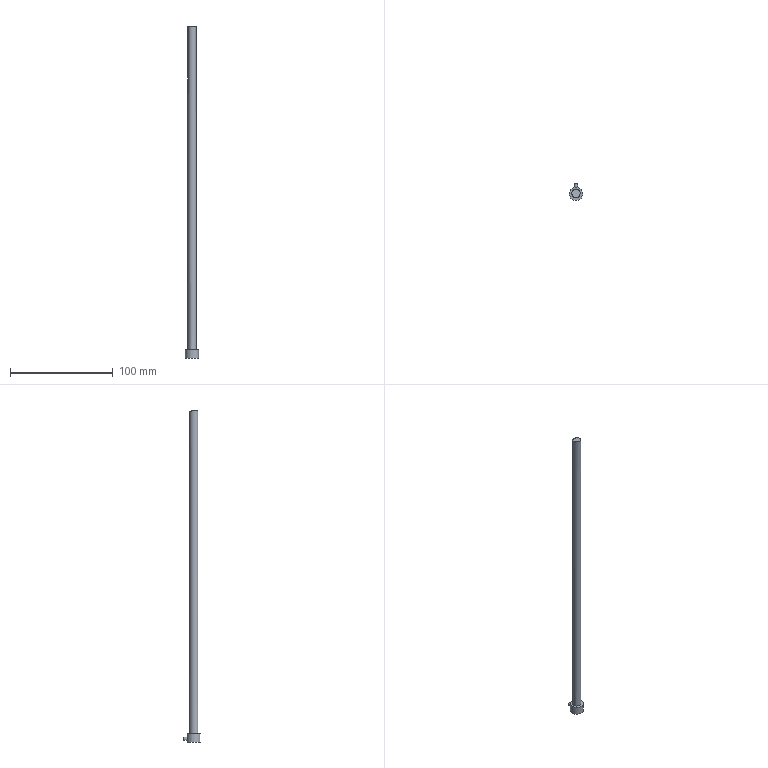Part | STEP file | E108-04-325 | 1 solid | 8 faces | box 13 x 16.5 x 322.523 mm | volume 16862 mm3 | cylinder 3 | plane 3 | spline 1 | cone 1 | commonest cylinder face diameters 3 x1 8 x1 13 x1
STEP:
#1=CARTESIAN_POINT('',(0.,0.,0.));
#2=DIRECTION('',(0.,0.,1.));
#3=DIRECTION('',(1.,0.,0.));
#4=AXIS2_PLACEMENT_3D('',#1,#2,#3);
#5=CARTESIAN_POINT('',(-1.397,3.748,321.27));
#6=VERTEX_POINT('',#5);
#7=CARTESIAN_POINT('',(-1.397,3.748,321.27));
#8=CARTESIAN_POINT('',(-1.815,3.592,321.278));
#9=CARTESIAN_POINT('',(-2.211,3.363,321.295));
#10=CARTESIAN_POINT('',(-2.554,3.079,321.322));
#11=CARTESIAN_POINT('',(-2.896,2.795,321.348));
#12=CARTESIAN_POINT('',(-3.194,2.449,321.384));
#13=CARTESIAN_POINT('',(-3.423,2.069,321.427));
#14=CARTESIAN_POINT('',(-3.653,1.688,321.472));
#15=CARTESIAN_POINT('',(-3.821,1.264,321.525));
#16=CARTESIAN_POINT('',(-3.913,0.83,321.584));
#17=CARTESIAN_POINT('',(-4.006,0.3925,321.644));
#18=CARTESIAN_POINT('',(-4.024,-0.06598,321.712));
#19=CARTESIAN_POINT('',(-3.968,-0.5081,321.783));
#20=CARTESIAN_POINT('',(-3.91,-0.955,321.854));
#21=CARTESIAN_POINT('',(-3.775,-1.397,321.93));
#22=CARTESIAN_POINT('',(-3.572,-1.8,322.004));
#23=CARTESIAN_POINT('',(-3.368,-2.204,322.078));
#24=CARTESIAN_POINT('',(-3.091,-2.58,322.152));
#25=CARTESIAN_POINT('',(-2.762,-2.893,322.219));
#26=CARTESIAN_POINT('',(-2.434,-3.207,322.285));
#27=CARTESIAN_POINT('',(-2.046,-3.467,322.346));
#28=CARTESIAN_POINT('',(-1.629,-3.653,322.394));
#29=CARTESIAN_POINT('',(-1.219,-3.836,322.442));
#30=CARTESIAN_POINT('',(-0.7694,-3.951,322.478));
#31=CARTESIAN_POINT('',(-0.3192,-3.987,322.499));
#32=CARTESIAN_POINT('',(0.123,-4.023,322.52));
#33=CARTESIAN_POINT('',(0.5783,-3.983,322.527));
#34=CARTESIAN_POINT('',(1.008,-3.871,322.519));
#35=CARTESIAN_POINT('',(1.434,-3.76,322.512));
#36=CARTESIAN_POINT('',(1.846,-3.576,322.489));
#37=CARTESIAN_POINT('',(2.211,-3.333,322.455));
#38=CARTESIAN_POINT('',(2.578,-3.09,322.421));
#39=CARTESIAN_POINT('',(2.907,-2.782,322.374));
#40=CARTESIAN_POINT('',(3.174,-2.434,322.319));
#41=CARTESIAN_POINT('',(3.444,-2.082,322.264));
#42=CARTESIAN_POINT('',(3.657,-1.679,322.199));
#43=CARTESIAN_POINT('',(3.797,-1.259,322.132));
#44=CARTESIAN_POINT('',(3.938,-0.8318,322.064));
#45=CARTESIAN_POINT('',(4.008,-0.3752,321.991));
#46=CARTESIAN_POINT('',(3.999,0.07396,321.92));
#47=CARTESIAN_POINT('',(3.991,0.5268,321.849));
#48=CARTESIAN_POINT('',(3.903,0.9847,321.778));
#49=CARTESIAN_POINT('',(3.743,1.409,321.712));
#50=CARTESIAN_POINT('',(3.584,1.833,321.647));
#51=CARTESIAN_POINT('',(3.348,2.236,321.585));
#52=CARTESIAN_POINT('',(3.054,2.583,321.531));
#53=CARTESIAN_POINT('',(2.763,2.928,321.478));
#54=CARTESIAN_POINT('',(2.406,3.227,321.431));
#55=CARTESIAN_POINT('',(2.015,3.455,321.393));
#56=CARTESIAN_POINT('',(1.628,3.681,321.355));
#57=CARTESIAN_POINT('',(1.195,3.844,321.324));
#58=CARTESIAN_POINT('',(0.7533,3.928,321.303));
#59=CARTESIAN_POINT('',(0.3148,4.013,321.282));
#60=CARTESIAN_POINT('',(-0.1448,4.022,321.27));
#61=CARTESIAN_POINT('',(-0.587,3.957,321.266));
#62=CARTESIAN_POINT('',(-0.8629,3.916,321.264));
#63=CARTESIAN_POINT('',(-1.136,3.845,321.265));
#64=CARTESIAN_POINT('',(-1.397,3.748,321.27));
#65=B_SPLINE_CURVE_WITH_KNOTS('',3,(#7,#8,#9,#10,#11,#12,#13,#14,#15,#16,#17,#18,#19,#20,#21,#22,#23,#24,#25,#26,#27,#28,#29,#30,#31,#32,#33,#34,#35,#36,#37,#38,#39,#40,#41,#42,#43,#44,#45,#46,#47,#48,#49,#50,#51,#52,#53,#54,#55,#56,#57,#58,#59,#60,#61,#62,#63,#64),.UNSPECIFIED.,.T.,.F.,(1,3,3,3,3,3,3,3,3,3,3,3,3,3,3,3,3,3,3,3,3,1),(-0.03296,0.,0.05312,0.1062,0.1595,0.2133,0.2677,0.3225,0.3772,0.4311,0.484,0.5364,0.589,0.6424,0.6966,0.7513,0.8059,0.8601,0.9138,0.967,1.,1.053),.UNSPECIFIED.);
#66=CARTESIAN_POINT('',(0.,0.,108.));
#67=DIRECTION('',(0.,0.,-1.));
#68=DIRECTION('',(-1.,0.,0.));
#69=AXIS2_PLACEMENT_3D('',#66,#67,#68);
#70=CYLINDRICAL_SURFACE('',#69,4.);
#71=CARTESIAN_POINT('',(7.497,-213.27));
#72=CARTESIAN_POINT('',(7.473,-213.272));
#73=CARTESIAN_POINT('',(7.426,-213.276));
#74=CARTESIAN_POINT('',(7.354,-213.285));
#75=CARTESIAN_POINT('',(7.282,-213.297));
#76=CARTESIAN_POINT('',(7.21,-213.31));
#77=CARTESIAN_POINT('',(7.138,-213.327));
#78=CARTESIAN_POINT('',(7.067,-213.346));
#79=CARTESIAN_POINT('',(6.995,-213.367));
#80=CARTESIAN_POINT('',(6.923,-213.391));
#81=CARTESIAN_POINT('',(6.852,-213.417));
#82=CARTESIAN_POINT('',(6.781,-213.446));
#83=CARTESIAN_POINT('',(6.709,-213.477));
#84=CARTESIAN_POINT('',(6.637,-213.51));
#85=CARTESIAN_POINT('',(6.566,-213.545));
#86=CARTESIAN_POINT('',(6.495,-213.583));
#87=CARTESIAN_POINT('',(6.424,-213.622));
#88=CARTESIAN_POINT('',(6.353,-213.662));
#89=CARTESIAN_POINT('',(6.282,-213.705));
#90=CARTESIAN_POINT('',(6.21,-213.748));
#91=CARTESIAN_POINT('',(6.14,-213.793));
#92=CARTESIAN_POINT('',(6.069,-213.838));
#93=CARTESIAN_POINT('',(5.998,-213.884));
#94=CARTESIAN_POINT('',(5.927,-213.931));
#95=CARTESIAN_POINT('',(5.856,-213.978));
#96=CARTESIAN_POINT('',(5.785,-214.024));
#97=CARTESIAN_POINT('',(5.715,-214.07));
#98=CARTESIAN_POINT('',(5.643,-214.116));
#99=CARTESIAN_POINT('',(5.572,-214.16));
#100=CARTESIAN_POINT('',(5.501,-214.203));
#101=CARTESIAN_POINT('',(5.431,-214.244));
#102=CARTESIAN_POINT('',(5.359,-214.284));
#103=CARTESIAN_POINT('',(5.288,-214.322));
#104=CARTESIAN_POINT('',(5.217,-214.357));
#105=CARTESIAN_POINT('',(5.145,-214.389));
#106=CARTESIAN_POINT('',(5.074,-214.418));
#107=CARTESIAN_POINT('',(5.003,-214.444));
#108=CARTESIAN_POINT('',(4.931,-214.467));
#109=CARTESIAN_POINT('',(4.859,-214.486));
#110=CARTESIAN_POINT('',(4.788,-214.501));
#111=CARTESIAN_POINT('',(4.716,-214.512));
#112=CARTESIAN_POINT('',(4.644,-214.52));
#113=CARTESIAN_POINT('',(4.572,-214.523));
#114=CARTESIAN_POINT('',(4.5,-214.522));
#115=CARTESIAN_POINT('',(4.429,-214.518));
#116=CARTESIAN_POINT('',(4.357,-214.509));
#117=CARTESIAN_POINT('',(4.285,-214.496));
#118=CARTESIAN_POINT('',(4.213,-214.48));
#119=CARTESIAN_POINT('',(4.141,-214.46));
#120=CARTESIAN_POINT('',(4.07,-214.437));
#121=CARTESIAN_POINT('',(3.998,-214.41));
#122=CARTESIAN_POINT('',(3.927,-214.381));
#123=CARTESIAN_POINT('',(3.855,-214.348));
#124=CARTESIAN_POINT('',(3.784,-214.314));
#125=CARTESIAN_POINT('',(3.713,-214.277));
#126=CARTESIAN_POINT('',(3.642,-214.238));
#127=CARTESIAN_POINT('',(3.57,-214.197));
#128=CARTESIAN_POINT('',(3.499,-214.155));
#129=CARTESIAN_POINT('',(3.429,-214.112));
#130=CARTESIAN_POINT('',(3.358,-214.068));
#131=CARTESIAN_POINT('',(3.286,-214.024));
#132=CARTESIAN_POINT('',(3.215,-213.979));
#133=CARTESIAN_POINT('',(3.144,-213.934));
#134=CARTESIAN_POINT('',(3.074,-213.889));
#135=CARTESIAN_POINT('',(3.003,-213.845));
#136=CARTESIAN_POINT('',(2.932,-213.801));
#137=CARTESIAN_POINT('',(2.86,-213.758));
#138=CARTESIAN_POINT('',(2.79,-213.717));
#139=CARTESIAN_POINT('',(2.719,-213.676));
#140=CARTESIAN_POINT('',(2.647,-213.637));
#141=CARTESIAN_POINT('',(2.576,-213.599));
#142=CARTESIAN_POINT('',(2.505,-213.563));
#143=CARTESIAN_POINT('',(2.434,-213.528));
#144=CARTESIAN_POINT('',(2.362,-213.496));
#145=CARTESIAN_POINT('',(2.291,-213.465));
#146=CARTESIAN_POINT('',(2.219,-213.436));
#147=CARTESIAN_POINT('',(2.148,-213.409));
#148=CARTESIAN_POINT('',(2.076,-213.385));
#149=CARTESIAN_POINT('',(2.005,-213.362));
#150=CARTESIAN_POINT('',(1.933,-213.342));
#151=CARTESIAN_POINT('',(1.861,-213.324));
#152=CARTESIAN_POINT('',(1.79,-213.309));
#153=CARTESIAN_POINT('',(1.718,-213.295));
#154=CARTESIAN_POINT('',(1.646,-213.284));
#155=CARTESIAN_POINT('',(1.574,-213.276));
#156=CARTESIAN_POINT('',(1.502,-213.27));
#157=CARTESIAN_POINT('',(1.431,-213.266));
#158=CARTESIAN_POINT('',(1.359,-213.265));
#159=CARTESIAN_POINT('',(1.286,-213.266));
#160=CARTESIAN_POINT('',(1.238,-213.269));
#161=CARTESIAN_POINT('',(1.214,-213.27));
#162=B_SPLINE_CURVE_WITH_KNOTS('',3,(#71,#72,#73,#74,#75,#76,#77,#78,#79,#80,#81,#82,#83,#84,#85,#86,#87,#88,#89,#90,#91,#92,#93,#94,#95,#96,#97,#98,#99,#100,#101,#102,#103,#104,#105,#106,#107,#108,#109,#110,#111,#112,#113,#114,#115,#116,#117,#118,#119,#120,#121,#122,#123,#124,#125,#126,#127,#128,#129,#130,#131,#132,#133,#134,#135,#136,#137,#138,#139,#140,#141,#142,#143,#144,#145,#146,#147,#148,#149,#150,#151,#152,#153,#154,#155,#156,#157,#158,#159,#160,#161),.UNSPECIFIED.,.F.,.F.,(4,1,1,1,1,1,1,1,1,1,1,1,1,1,1,1,1,1,1,1,1,1,1,1,1,1,1,1,1,1,1,1,1,1,1,1,1,1,1,1,1,1,1,1,1,1,1,1,1,1,1,1,1,1,1,1,1,1,1,1,1,1,1,1,1,1,1,1,1,1,1,1,1,1,1,1,1,1,1,1,1,1,1,1,1,1,1,1,4),(0.,0.01136,0.02273,0.03409,0.04545,0.05682,0.06818,0.07955,0.09091,0.1023,0.1136,0.125,0.1364,0.1477,0.1591,0.1705,0.1818,0.1932,0.2045,0.2159,0.2273,0.2386,0.25,0.2614,0.2727,0.2841,0.2955,0.3068,0.3182,0.3295,0.3409,0.3523,0.3636,0.375,0.3864,0.3977,0.4091,0.4205,0.4318,0.4432,0.4545,0.4659,0.4773,0.4886,0.5,0.5114,0.5227,0.5341,0.5455,0.5568,0.5682,0.5795,0.5909,0.6023,0.6136,0.625,0.6364,0.6477,0.6591,0.6705,0.6818,0.6932,0.7045,0.7159,0.7273,0.7386,0.75,0.7614,0.7727,0.7841,0.7955,0.8068,0.8182,0.8295,0.8409,0.8523,0.8636,0.875,0.8864,0.8977,0.9091,0.9205,0.9318,0.9432,0.9545,0.9659,0.9773,0.9886,1.),.QUASI_UNIFORM_KNOTS.);
#163=(GEOMETRIC_REPRESENTATION_CONTEXT(2)PARAMETRIC_REPRESENTATION_CONTEXT()REPRESENTATION_CONTEXT('',''));
#164=DEFINITIONAL_REPRESENTATION('',(#162),#163);
#165=PCURVE('',#70,#164);
#166=CARTESIAN_POINT('',(19.927,-1.061,321.866));
#167=CARTESIAN_POINT('',(18.638,5.204,320.799));
#168=CARTESIAN_POINT('',(17.382,11.513,320.097));
#169=CARTESIAN_POINT('',(16.146,17.876,319.645));
#170=CARTESIAN_POINT('',(13.703,-2.125,322.326));
#171=CARTESIAN_POINT('',(12.375,4.073,321.242));
#172=CARTESIAN_POINT('',(11.072,10.308,320.518));
#173=CARTESIAN_POINT('',(9.785,16.592,320.042));
#174=CARTESIAN_POINT('',(7.218,-3.361,322.621));
#175=CARTESIAN_POINT('',(5.852,2.773,321.508));
#176=CARTESIAN_POINT('',(4.506,8.942,320.75));
#177=CARTESIAN_POINT('',(3.17,15.156,320.239));
#178=CARTESIAN_POINT('',(-6.604,-6.202,322.705));
#179=CARTESIAN_POINT('',(-8.034,-0.1978,321.507));
#180=CARTESIAN_POINT('',(-9.458,5.839,320.656));
#181=CARTESIAN_POINT('',(-10.883,11.916,320.054));
#182=CARTESIAN_POINT('',(-13.939,-7.81,322.49));
#183=CARTESIAN_POINT('',(-15.395,-1.87,321.235));
#184=CARTESIAN_POINT('',(-16.854,4.101,320.327));
#185=CARTESIAN_POINT('',(-18.32,10.11,319.669));
#186=CARTESIAN_POINT('',(-29.513,-11.391,321.285));
#187=CARTESIAN_POINT('',(-31.002,-5.589,319.888));
#188=CARTESIAN_POINT('',(-32.516,0.2464,318.841));
#189=CARTESIAN_POINT('',(-34.052,6.11,318.053));
#190=CARTESIAN_POINT('',(-37.747,-13.364,320.293));
#191=CARTESIAN_POINT('',(-39.245,-7.634,318.809));
#192=CARTESIAN_POINT('',(-40.779,-1.871,317.681));
#193=CARTESIAN_POINT('',(-42.344,3.916,316.819));
#194=CARTESIAN_POINT('',(-54.974,-17.604,317.285));
#195=CARTESIAN_POINT('',(-56.464,-12.039,315.613));
#196=CARTESIAN_POINT('',(-58.018,-6.437,314.309));
#197=CARTESIAN_POINT('',(-59.625,-0.8214,313.287));
#198=CARTESIAN_POINT('',(-63.963,-19.87,315.268));
#199=CARTESIAN_POINT('',(-65.438,-14.397,313.494));
#200=CARTESIAN_POINT('',(-66.991,-8.885,312.095));
#201=CARTESIAN_POINT('',(-68.61,-3.364,310.987));
#202=CARTESIAN_POINT('',(-73.219,-22.228,312.641));
#203=CARTESIAN_POINT('',(-74.668,-16.858,310.779));
#204=CARTESIAN_POINT('',(-76.208,-11.45,309.295));
#205=CARTESIAN_POINT('',(-77.828,-6.035,308.108));
#206=B_SPLINE_SURFACE_WITH_KNOTS('',3,3,((#166,#167,#168,#169),(#170,#171,#172,#173),(#174,#175,#176,#177),(#178,#179,#180,#181),(#182,#183,#184,#185),(#186,#187,#188,#189),(#190,#191,#192,#193),(#194,#195,#196,#197),(#198,#199,#200,#201),(#202,#203,#204,#205)),.UNSPECIFIED.,.F.,.F.,.F.,(4,2,2,2,4),(4,4),(0.,0.25,0.5,0.75,1.),(0.,1.),.UNSPECIFIED.);
#207=CARTESIAN_POINT('',(0.2472,0.4644));
#208=CARTESIAN_POINT('',(0.2483,0.4637));
#209=CARTESIAN_POINT('',(0.2505,0.4619));
#210=CARTESIAN_POINT('',(0.2538,0.458));
#211=CARTESIAN_POINT('',(0.257,0.4532));
#212=CARTESIAN_POINT('',(0.2601,0.4473));
#213=CARTESIAN_POINT('',(0.2631,0.4405));
#214=CARTESIAN_POINT('',(0.2659,0.4326));
#215=CARTESIAN_POINT('',(0.2687,0.4239));
#216=CARTESIAN_POINT('',(0.2713,0.4142));
#217=CARTESIAN_POINT('',(0.2738,0.4038));
#218=CARTESIAN_POINT('',(0.276,0.3926));
#219=CARTESIAN_POINT('',(0.2781,0.3807));
#220=CARTESIAN_POINT('',(0.28,0.3681));
#221=CARTESIAN_POINT('',(0.2817,0.3549));
#222=CARTESIAN_POINT('',(0.2833,0.3413));
#223=CARTESIAN_POINT('',(0.2845,0.3272));
#224=CARTESIAN_POINT('',(0.2856,0.3127));
#225=CARTESIAN_POINT('',(0.2865,0.2979));
#226=CARTESIAN_POINT('',(0.2871,0.2829));
#227=CARTESIAN_POINT('',(0.2875,0.2679));
#228=CARTESIAN_POINT('',(0.2876,0.2527));
#229=CARTESIAN_POINT('',(0.2876,0.2374));
#230=CARTESIAN_POINT('',(0.2873,0.2223));
#231=CARTESIAN_POINT('',(0.2867,0.2073));
#232=CARTESIAN_POINT('',(0.286,0.1926));
#233=CARTESIAN_POINT('',(0.285,0.1782));
#234=CARTESIAN_POINT('',(0.2838,0.1641));
#235=CARTESIAN_POINT('',(0.2824,0.1505));
#236=CARTESIAN_POINT('',(0.2807,0.1374));
#237=CARTESIAN_POINT('',(0.2789,0.1249));
#238=CARTESIAN_POINT('',(0.2769,0.113));
#239=CARTESIAN_POINT('',(0.2747,0.1018));
#240=CARTESIAN_POINT('',(0.2723,0.0914));
#241=CARTESIAN_POINT('',(0.2697,0.08183));
#242=CARTESIAN_POINT('',(0.267,0.07317));
#243=CARTESIAN_POINT('',(0.2641,0.06539));
#244=CARTESIAN_POINT('',(0.2612,0.05855));
#245=CARTESIAN_POINT('',(0.2581,0.05272));
#246=CARTESIAN_POINT('',(0.2549,0.04796));
#247=CARTESIAN_POINT('',(0.2516,0.04427));
#248=CARTESIAN_POINT('',(0.2483,0.04165));
#249=CARTESIAN_POINT('',(0.2449,0.04012));
#250=CARTESIAN_POINT('',(0.2415,0.0397));
#251=CARTESIAN_POINT('',(0.2381,0.04039));
#252=CARTESIAN_POINT('',(0.2347,0.0422));
#253=CARTESIAN_POINT('',(0.2313,0.04511));
#254=CARTESIAN_POINT('',(0.228,0.04908));
#255=CARTESIAN_POINT('',(0.2247,0.05408));
#256=CARTESIAN_POINT('',(0.2216,0.06009));
#257=CARTESIAN_POINT('',(0.2185,0.06713));
#258=CARTESIAN_POINT('',(0.2155,0.07511));
#259=CARTESIAN_POINT('',(0.2127,0.08397));
#260=CARTESIAN_POINT('',(0.21,0.09363));
#261=CARTESIAN_POINT('',(0.2075,0.1041));
#262=CARTESIAN_POINT('',(0.2051,0.1154));
#263=CARTESIAN_POINT('',(0.2029,0.1273));
#264=CARTESIAN_POINT('',(0.2009,0.1399));
#265=CARTESIAN_POINT('',(0.1992,0.1529));
#266=CARTESIAN_POINT('',(0.1976,0.1665));
#267=CARTESIAN_POINT('',(0.1963,0.1805));
#268=CARTESIAN_POINT('',(0.1952,0.1949));
#269=CARTESIAN_POINT('',(0.1943,0.2096));
#270=CARTESIAN_POINT('',(0.1936,0.2244));
#271=CARTESIAN_POINT('',(0.1933,0.2394));
#272=CARTESIAN_POINT('',(0.1931,0.2545));
#273=CARTESIAN_POINT('',(0.1932,0.2696));
#274=CARTESIAN_POINT('',(0.1935,0.2846));
#275=CARTESIAN_POINT('',(0.1941,0.2993));
#276=CARTESIAN_POINT('',(0.1949,0.314));
#277=CARTESIAN_POINT('',(0.196,0.3283));
#278=CARTESIAN_POINT('',(0.1972,0.3423));
#279=CARTESIAN_POINT('',(0.1987,0.3558));
#280=CARTESIAN_POINT('',(0.2005,0.3688));
#281=CARTESIAN_POINT('',(0.2024,0.3812));
#282=CARTESIAN_POINT('',(0.2045,0.3931));
#283=CARTESIAN_POINT('',(0.2068,0.4042));
#284=CARTESIAN_POINT('',(0.2093,0.4145));
#285=CARTESIAN_POINT('',(0.2119,0.424));
#286=CARTESIAN_POINT('',(0.2147,0.4327));
#287=CARTESIAN_POINT('',(0.2177,0.4405));
#288=CARTESIAN_POINT('',(0.2207,0.4474));
#289=CARTESIAN_POINT('',(0.2238,0.4532));
#290=CARTESIAN_POINT('',(0.227,0.458));
#291=CARTESIAN_POINT('',(0.2303,0.4618));
#292=CARTESIAN_POINT('',(0.2337,0.4646));
#293=CARTESIAN_POINT('',(0.237,0.4662));
#294=CARTESIAN_POINT('',(0.2404,0.4668));
#295=CARTESIAN_POINT('',(0.2438,0.4662));
#296=CARTESIAN_POINT('',(0.2461,0.4651));
#297=CARTESIAN_POINT('',(0.2472,0.4644));
#298=B_SPLINE_CURVE_WITH_KNOTS('',3,(#207,#208,#209,#210,#211,#212,#213,#214,#215,#216,#217,#218,#219,#220,#221,#222,#223,#224,#225,#226,#227,#228,#229,#230,#231,#232,#233,#234,#235,#236,#237,#238,#239,#240,#241,#242,#243,#244,#245,#246,#247,#248,#249,#250,#251,#252,#253,#254,#255,#256,#257,#258,#259,#260,#261,#262,#263,#264,#265,#266,#267,#268,#269,#270,#271,#272,#273,#274,#275,#276,#277,#278,#279,#280,#281,#282,#283,#284,#285,#286,#287,#288,#289,#290,#291,#292,#293,#294,#295,#296,#297),.UNSPECIFIED.,.T.,.F.,(4,1,1,1,1,1,1,1,1,1,1,1,1,1,1,1,1,1,1,1,1,1,1,1,1,1,1,1,1,1,1,1,1,1,1,1,1,1,1,1,1,1,1,1,1,1,1,1,1,1,1,1,1,1,1,1,1,1,1,1,1,1,1,1,1,1,1,1,1,1,1,1,1,1,1,1,1,1,1,1,1,1,1,1,1,1,1,1,4),(0.,0.01136,0.02273,0.03409,0.04545,0.05682,0.06818,0.07955,0.09091,0.1023,0.1136,0.125,0.1364,0.1477,0.1591,0.1705,0.1818,0.1932,0.2045,0.2159,0.2273,0.2386,0.25,0.2614,0.2727,0.2841,0.2955,0.3068,0.3182,0.3295,0.3409,0.3523,0.3636,0.375,0.3864,0.3977,0.4091,0.4205,0.4318,0.4432,0.4545,0.4659,0.4773,0.4886,0.5,0.5114,0.5227,0.5341,0.5455,0.5568,0.5682,0.5795,0.5909,0.6023,0.6136,0.625,0.6364,0.6477,0.6591,0.6705,0.6818,0.6932,0.7045,0.7159,0.7273,0.7386,0.75,0.7614,0.7727,0.7841,0.7955,0.8068,0.8182,0.8295,0.8409,0.8523,0.8636,0.875,0.8864,0.8977,0.9091,0.9205,0.9318,0.9432,0.9545,0.9659,0.9773,0.9886,1.),.QUASI_UNIFORM_KNOTS.);
#299=(GEOMETRIC_REPRESENTATION_CONTEXT(2)PARAMETRIC_REPRESENTATION_CONTEXT()REPRESENTATION_CONTEXT('',''));
#300=DEFINITIONAL_REPRESENTATION('',(#298),#299);
#301=PCURVE('',#206,#300);
#302=SURFACE_CURVE('',#65,(#165,#301),.PCURVE_S1.);
#303=EDGE_CURVE('',#6,#6,#302,.T.);
#304=ORIENTED_EDGE('',*,*,#303,.F.);
#305=CARTESIAN_POINT('',(-1.397,3.748,8.));
#306=VERTEX_POINT('',#305);
#307=CARTESIAN_POINT('',(-1.397,3.748,321.27));
#308=CARTESIAN_POINT('',(-1.397,3.748,8.));
#309=B_SPLINE_CURVE_WITH_KNOTS('',1,(#307,#308),.UNSPECIFIED.,.F.,.F.,(2,2),(-213.27,100.),.PIECEWISE_BEZIER_KNOTS.);
#310=CARTESIAN_POINT('',(7.497,0.));
#311=DIRECTION('',(0.,1.));
#312=VECTOR('',#311,1.);
#313=LINE('',#310,#312);
#314=(GEOMETRIC_REPRESENTATION_CONTEXT(2)PARAMETRIC_REPRESENTATION_CONTEXT()REPRESENTATION_CONTEXT('',''));
#315=DEFINITIONAL_REPRESENTATION('',(#313),#314);
#316=PCURVE('',#70,#315);
#317=CARTESIAN_POINT('',(1.214,0.));
#318=DIRECTION('',(0.,1.));
#319=VECTOR('',#318,1.);
#320=LINE('',#317,#319);
#321=(GEOMETRIC_REPRESENTATION_CONTEXT(2)PARAMETRIC_REPRESENTATION_CONTEXT()REPRESENTATION_CONTEXT('',''));
#322=DEFINITIONAL_REPRESENTATION('',(#320),#321);
#323=PCURVE('',#70,#322);
#324=SEAM_CURVE('',#309,(#316,#323),.PCURVE_S1.);
#325=EDGE_CURVE('',#6,#306,#324,.T.);
#326=ORIENTED_EDGE('',*,*,#325,.T.);
#327=CARTESIAN_POINT('',(4.,0.,8.));
#328=VERTEX_POINT('',#327);
#329=CARTESIAN_POINT('',(0.,0.,8.));
#330=DIRECTION('',(0.,0.,1.));
#331=DIRECTION('',(1.,0.,0.));
#332=AXIS2_PLACEMENT_3D('',#329,#330,#331);
#333=CIRCLE('',#332,4.);
#334=CARTESIAN_POINT('',(9.425,100.));
#335=DIRECTION('',(-1.,0.));
#336=VECTOR('',#335,1.);
#337=LINE('',#334,#336);
#338=(GEOMETRIC_REPRESENTATION_CONTEXT(2)PARAMETRIC_REPRESENTATION_CONTEXT()REPRESENTATION_CONTEXT('',''));
#339=DEFINITIONAL_REPRESENTATION('',(#337),#338);
#340=PCURVE('',#70,#339);
#341=CARTESIAN_POINT('',(0.,0.,8.));
#342=DIRECTION('',(0.,0.,-1.));
#343=DIRECTION('',(1.,0.,0.));
#344=AXIS2_PLACEMENT_3D('',#341,#342,#343);
#345=PLANE('',#344);
#346=CARTESIAN_POINT('',(4.,0.));
#347=CARTESIAN_POINT('',(4.,-6.928));
#348=CARTESIAN_POINT('',(-2.,-3.464));
#349=CARTESIAN_POINT('',(-8.,0.));
#350=CARTESIAN_POINT('',(-2.,3.464));
#351=CARTESIAN_POINT('',(4.,6.928));
#352=CARTESIAN_POINT('',(4.,0.));
#353=(BOUNDED_CURVE()B_SPLINE_CURVE(2,(#346,#347,#348,#349,#350,#351,#352),.UNSPECIFIED.,.T.,.F.)B_SPLINE_CURVE_WITH_KNOTS((1,2,2,2,2,1),(-2.094,0.,2.094,4.189,6.283,8.378),.UNSPECIFIED.)CURVE()GEOMETRIC_REPRESENTATION_ITEM()RATIONAL_B_SPLINE_CURVE((1.,0.5,1.,0.5,1.,0.5,1.))REPRESENTATION_ITEM(''));
#354=(GEOMETRIC_REPRESENTATION_CONTEXT(2)PARAMETRIC_REPRESENTATION_CONTEXT()REPRESENTATION_CONTEXT('',''));
#355=DEFINITIONAL_REPRESENTATION('',(#353),#354);
#356=PCURVE('',#345,#355);
#357=SURFACE_CURVE('',#333,(#340,#356),.PCURVE_S1.);
#358=EDGE_CURVE('',#306,#328,#357,.T.);
#359=ORIENTED_EDGE('',*,*,#358,.T.);
#360=CARTESIAN_POINT('',(0.,0.,8.));
#361=DIRECTION('',(0.,0.,1.));
#362=DIRECTION('',(1.,0.,0.));
#363=AXIS2_PLACEMENT_3D('',#360,#361,#362);
#364=CIRCLE('',#363,4.);
#365=CARTESIAN_POINT('',(3.142,100.));
#366=DIRECTION('',(-1.,0.));
#367=VECTOR('',#366,1.);
#368=LINE('',#365,#367);
#369=(GEOMETRIC_REPRESENTATION_CONTEXT(2)PARAMETRIC_REPRESENTATION_CONTEXT()REPRESENTATION_CONTEXT('',''));
#370=DEFINITIONAL_REPRESENTATION('',(#368),#369);
#371=PCURVE('',#70,#370);
#372=CARTESIAN_POINT('',(4.,0.));
#373=CARTESIAN_POINT('',(4.,-6.928));
#374=CARTESIAN_POINT('',(-2.,-3.464));
#375=CARTESIAN_POINT('',(-8.,0.));
#376=CARTESIAN_POINT('',(-2.,3.464));
#377=CARTESIAN_POINT('',(4.,6.928));
#378=CARTESIAN_POINT('',(4.,0.));
#379=(BOUNDED_CURVE()B_SPLINE_CURVE(2,(#372,#373,#374,#375,#376,#377,#378),.UNSPECIFIED.,.T.,.F.)B_SPLINE_CURVE_WITH_KNOTS((1,2,2,2,2,1),(-2.094,0.,2.094,4.189,6.283,8.378),.UNSPECIFIED.)CURVE()GEOMETRIC_REPRESENTATION_ITEM()RATIONAL_B_SPLINE_CURVE((1.,0.5,1.,0.5,1.,0.5,1.))REPRESENTATION_ITEM(''));
#380=(GEOMETRIC_REPRESENTATION_CONTEXT(2)PARAMETRIC_REPRESENTATION_CONTEXT()REPRESENTATION_CONTEXT('',''));
#381=DEFINITIONAL_REPRESENTATION('',(#379),#380);
#382=PCURVE('',#345,#381);
#383=SURFACE_CURVE('',#364,(#371,#382),.PCURVE_S1.);
#384=EDGE_CURVE('',#328,#306,#383,.T.);
#385=ORIENTED_EDGE('',*,*,#384,.T.);
#386=ORIENTED_EDGE('',*,*,#325,.F.);
#387=EDGE_LOOP('',(#304,#326,#359,#385,#386));
#388=FACE_BOUND('',#387,.T.);
#389=ADVANCED_FACE('',(#388),#70,.T.);
#390=ORIENTED_EDGE('',*,*,#303,.F.);
#391=EDGE_LOOP('',(#390));
#392=FACE_BOUND('',#391,.F.);
#393=ADVANCED_FACE('',(#392),#206,.F.);
#394=CARTESIAN_POINT('',(6.5,0.,0.));
#395=VERTEX_POINT('',#394);
#396=CARTESIAN_POINT('',(-6.5,0.,0.));
#397=VERTEX_POINT('',#396);
#398=CARTESIAN_POINT('',(0.,0.,0.));
#399=DIRECTION('',(0.,0.,-1.));
#400=DIRECTION('',(-1.,0.,0.));
#401=AXIS2_PLACEMENT_3D('',#398,#399,#400);
#402=CIRCLE('',#401,6.5);
#403=CARTESIAN_POINT('',(0.,0.,8.));
#404=DIRECTION('',(0.,0.,-1.));
#405=DIRECTION('',(1.,0.,0.));
#406=AXIS2_PLACEMENT_3D('',#403,#404,#405);
#407=CYLINDRICAL_SURFACE('',#406,6.5);
#408=CARTESIAN_POINT('',(-3.142,8.));
#409=DIRECTION('',(1.,0.));
#410=VECTOR('',#409,1.);
#411=LINE('',#408,#410);
#412=(GEOMETRIC_REPRESENTATION_CONTEXT(2)PARAMETRIC_REPRESENTATION_CONTEXT()REPRESENTATION_CONTEXT('',''));
#413=DEFINITIONAL_REPRESENTATION('',(#411),#412);
#414=PCURVE('',#407,#413);
#415=CARTESIAN_POINT('',(240.,-1000.,0.));
#416=DIRECTION('',(0.,0.,1.));
#417=DIRECTION('',(-1.,0.,0.));
#418=AXIS2_PLACEMENT_3D('',#415,#416,#417);
#419=PLANE('',#418);
#420=CARTESIAN_POINT('',(246.5,-1000.));
#421=CARTESIAN_POINT('',(246.5,-1011.258));
#422=CARTESIAN_POINT('',(236.75,-1005.629));
#423=CARTESIAN_POINT('',(227.,-1000.));
#424=CARTESIAN_POINT('',(236.75,-994.371));
#425=CARTESIAN_POINT('',(246.5,-988.742));
#426=CARTESIAN_POINT('',(246.5,-1000.));
#427=(BOUNDED_CURVE()B_SPLINE_CURVE(2,(#420,#421,#422,#423,#424,#425,#426),.UNSPECIFIED.,.T.,.F.)B_SPLINE_CURVE_WITH_KNOTS((1,2,2,2,2,1),(-2.094,0.,2.094,4.189,6.283,8.378),.UNSPECIFIED.)CURVE()GEOMETRIC_REPRESENTATION_ITEM()RATIONAL_B_SPLINE_CURVE((1.,0.5,1.,0.5,1.,0.5,1.))REPRESENTATION_ITEM(''));
#428=(GEOMETRIC_REPRESENTATION_CONTEXT(2)PARAMETRIC_REPRESENTATION_CONTEXT()REPRESENTATION_CONTEXT('',''));
#429=DEFINITIONAL_REPRESENTATION('',(#427),#428);
#430=PCURVE('',#419,#429);
#431=SURFACE_CURVE('',#402,(#414,#430),.PCURVE_S1.);
#432=EDGE_CURVE('',#395,#397,#431,.T.);
#433=ORIENTED_EDGE('',*,*,#432,.F.);
#434=CARTESIAN_POINT('',(6.5,0.,8.));
#435=VERTEX_POINT('',#434);
#436=CARTESIAN_POINT('',(6.5,0.,8.));
#437=CARTESIAN_POINT('',(6.5,0.,0.));
#438=B_SPLINE_CURVE_WITH_KNOTS('',1,(#436,#437),.UNSPECIFIED.,.F.,.F.,(2,2),(0.,8.),.PIECEWISE_BEZIER_KNOTS.);
#439=CARTESIAN_POINT('',(0.,0.));
#440=DIRECTION('',(0.,1.));
#441=VECTOR('',#440,1.);
#442=LINE('',#439,#441);
#443=(GEOMETRIC_REPRESENTATION_CONTEXT(2)PARAMETRIC_REPRESENTATION_CONTEXT()REPRESENTATION_CONTEXT('',''));
#444=DEFINITIONAL_REPRESENTATION('',(#442),#443);
#445=PCURVE('',#407,#444);
#446=CARTESIAN_POINT('',(6.283,0.));
#447=DIRECTION('',(0.,1.));
#448=VECTOR('',#447,1.);
#449=LINE('',#446,#448);
#450=(GEOMETRIC_REPRESENTATION_CONTEXT(2)PARAMETRIC_REPRESENTATION_CONTEXT()REPRESENTATION_CONTEXT('',''));
#451=DEFINITIONAL_REPRESENTATION('',(#449),#450);
#452=PCURVE('',#407,#451);
#453=SEAM_CURVE('',#438,(#445,#452),.PCURVE_S1.);
#454=EDGE_CURVE('',#435,#395,#453,.T.);
#455=ORIENTED_EDGE('',*,*,#454,.F.);
#456=CARTESIAN_POINT('',(0.,0.,8.));
#457=DIRECTION('',(0.,0.,-1.));
#458=DIRECTION('',(1.,0.,0.));
#459=AXIS2_PLACEMENT_3D('',#456,#457,#458);
#460=CIRCLE('',#459,6.5);
#461=CARTESIAN_POINT('',(0.,0.));
#462=DIRECTION('',(1.,0.));
#463=VECTOR('',#462,1.);
#464=LINE('',#461,#463);
#465=(GEOMETRIC_REPRESENTATION_CONTEXT(2)PARAMETRIC_REPRESENTATION_CONTEXT()REPRESENTATION_CONTEXT('',''));
#466=DEFINITIONAL_REPRESENTATION('',(#464),#465);
#467=PCURVE('',#407,#466);
#468=CARTESIAN_POINT('',(0.,0.));
#469=DIRECTION('',(1.,0.));
#470=AXIS2_PLACEMENT_2D('',#468,#469);
#471=CIRCLE('',#470,6.5);
#472=(GEOMETRIC_REPRESENTATION_CONTEXT(2)PARAMETRIC_REPRESENTATION_CONTEXT()REPRESENTATION_CONTEXT('',''));
#473=DEFINITIONAL_REPRESENTATION('',(#471),#472);
#474=PCURVE('',#345,#473);
#475=SURFACE_CURVE('',#460,(#467,#474),.PCURVE_S1.);
#476=EDGE_CURVE('',#435,#435,#475,.T.);
#477=ORIENTED_EDGE('',*,*,#476,.T.);
#478=ORIENTED_EDGE('',*,*,#454,.T.);
#479=CARTESIAN_POINT('',(0.,0.,0.));
#480=DIRECTION('',(0.,0.,-1.));
#481=DIRECTION('',(-1.,0.,0.));
#482=AXIS2_PLACEMENT_3D('',#479,#480,#481);
#483=CIRCLE('',#482,6.5);
#484=CARTESIAN_POINT('',(3.142,8.));
#485=DIRECTION('',(1.,0.));
#486=VECTOR('',#485,1.);
#487=LINE('',#484,#486);
#488=(GEOMETRIC_REPRESENTATION_CONTEXT(2)PARAMETRIC_REPRESENTATION_CONTEXT()REPRESENTATION_CONTEXT('',''));
#489=DEFINITIONAL_REPRESENTATION('',(#487),#488);
#490=PCURVE('',#407,#489);
#491=CARTESIAN_POINT('',(246.5,-1000.));
#492=CARTESIAN_POINT('',(246.5,-1011.258));
#493=CARTESIAN_POINT('',(236.75,-1005.629));
#494=CARTESIAN_POINT('',(227.,-1000.));
#495=CARTESIAN_POINT('',(236.75,-994.371));
#496=CARTESIAN_POINT('',(246.5,-988.742));
#497=CARTESIAN_POINT('',(246.5,-1000.));
#498=(BOUNDED_CURVE()B_SPLINE_CURVE(2,(#491,#492,#493,#494,#495,#496,#497),.UNSPECIFIED.,.T.,.F.)B_SPLINE_CURVE_WITH_KNOTS((1,2,2,2,2,1),(-2.094,0.,2.094,4.189,6.283,8.378),.UNSPECIFIED.)CURVE()GEOMETRIC_REPRESENTATION_ITEM()RATIONAL_B_SPLINE_CURVE((1.,0.5,1.,0.5,1.,0.5,1.))REPRESENTATION_ITEM(''));
#499=(GEOMETRIC_REPRESENTATION_CONTEXT(2)PARAMETRIC_REPRESENTATION_CONTEXT()REPRESENTATION_CONTEXT('',''));
#500=DEFINITIONAL_REPRESENTATION('',(#498),#499);
#501=PCURVE('',#419,#500);
#502=SURFACE_CURVE('',#483,(#490,#501),.PCURVE_S1.);
#503=EDGE_CURVE('',#397,#395,#502,.T.);
#504=ORIENTED_EDGE('',*,*,#503,.F.);
#505=EDGE_LOOP('',(#433,#455,#477,#478,#504));
#506=FACE_BOUND('',#505,.T.);
#507=CARTESIAN_POINT('',(0.,6.5,1.5));
#508=VERTEX_POINT('',#507);
#509=CARTESIAN_POINT('',(0.,6.5,1.5));
#510=CARTESIAN_POINT('',(0.1654,6.5,1.5));
#511=CARTESIAN_POINT('',(0.3332,6.493,1.528));
#512=CARTESIAN_POINT('',(0.4892,6.482,1.582));
#513=CARTESIAN_POINT('',(0.6451,6.47,1.636));
#514=CARTESIAN_POINT('',(0.7936,6.453,1.717));
#515=CARTESIAN_POINT('',(0.9231,6.434,1.818));
#516=CARTESIAN_POINT('',(1.055,6.415,1.92));
#517=CARTESIAN_POINT('',(1.17,6.394,2.047));
#518=CARTESIAN_POINT('',(1.261,6.377,2.187));
#519=CARTESIAN_POINT('',(1.352,6.358,2.329));
#520=CARTESIAN_POINT('',(1.421,6.343,2.49));
#521=CARTESIAN_POINT('',(1.46,6.334,2.655));
#522=CARTESIAN_POINT('',(1.498,6.325,2.817));
#523=CARTESIAN_POINT('',(1.509,6.322,2.989));
#524=CARTESIAN_POINT('',(1.492,6.326,3.155));
#525=CARTESIAN_POINT('',(1.475,6.33,3.318));
#526=CARTESIAN_POINT('',(1.431,6.341,3.48));
#527=CARTESIAN_POINT('',(1.362,6.356,3.628));
#528=CARTESIAN_POINT('',(1.293,6.37,3.777));
#529=CARTESIAN_POINT('',(1.199,6.39,3.917));
#530=CARTESIAN_POINT('',(1.085,6.409,4.035));
#531=CARTESIAN_POINT('',(0.9695,6.428,4.157));
#532=CARTESIAN_POINT('',(0.8309,6.448,4.26));
#533=CARTESIAN_POINT('',(0.6809,6.464,4.337));
#534=CARTESIAN_POINT('',(0.5305,6.48,4.413));
#535=CARTESIAN_POINT('',(0.3642,6.492,4.465));
#536=CARTESIAN_POINT('',(0.1962,6.497,4.487));
#537=CARTESIAN_POINT('',(0.03191,6.502,4.509));
#538=CARTESIAN_POINT('',(-0.1386,6.501,4.503));
#539=CARTESIAN_POINT('',(-0.3008,6.493,4.47));
#540=CARTESIAN_POINT('',(-0.4611,6.486,4.437));
#541=CARTESIAN_POINT('',(-0.6177,6.472,4.377));
#542=CARTESIAN_POINT('',(-0.7583,6.456,4.294));
#543=CARTESIAN_POINT('',(-0.9011,6.439,4.211));
#544=CARTESIAN_POINT('',(-1.031,6.419,4.102));
#545=CARTESIAN_POINT('',(-1.139,6.399,3.976));
#546=CARTESIAN_POINT('',(-1.249,6.38,3.848));
#547=CARTESIAN_POINT('',(-1.338,6.361,3.699));
#548=CARTESIAN_POINT('',(-1.399,6.348,3.541));
#549=CARTESIAN_POINT('',(-1.46,6.334,3.384));
#550=CARTESIAN_POINT('',(-1.494,6.326,3.214));
#551=CARTESIAN_POINT('',(-1.499,6.325,3.046));
#552=CARTESIAN_POINT('',(-1.504,6.324,2.881));
#553=CARTESIAN_POINT('',(-1.482,6.329,2.714));
#554=CARTESIAN_POINT('',(-1.433,6.34,2.557));
#555=CARTESIAN_POINT('',(-1.385,6.351,2.4));
#556=CARTESIAN_POINT('',(-1.309,6.367,2.25));
#557=CARTESIAN_POINT('',(-1.214,6.386,2.119));
#558=CARTESIAN_POINT('',(-1.116,6.404,1.984));
#559=CARTESIAN_POINT('',(-0.9937,6.425,1.864));
#560=CARTESIAN_POINT('',(-0.8569,6.443,1.769));
#561=CARTESIAN_POINT('',(-0.7182,6.462,1.672));
#562=CARTESIAN_POINT('',(-0.5604,6.478,1.598));
#563=CARTESIAN_POINT('',(-0.3967,6.488,1.553));
#564=CARTESIAN_POINT('',(-0.2682,6.496,1.518));
#565=CARTESIAN_POINT('',(-0.1335,6.5,1.5));
#566=CARTESIAN_POINT('',(0.,6.5,1.5));
#567=B_SPLINE_CURVE_WITH_KNOTS('',3,(#509,#510,#511,#512,#513,#514,#515,#516,#517,#518,#519,#520,#521,#522,#523,#524,#525,#526,#527,#528,#529,#530,#531,#532,#533,#534,#535,#536,#537,#538,#539,#540,#541,#542,#543,#544,#545,#546,#547,#548,#549,#550,#551,#552,#553,#554,#555,#556,#557,#558,#559,#560,#561,#562,#563,#564,#565,#566),.UNSPECIFIED.,.T.,.F.,(1,3,3,3,3,3,3,3,3,3,3,3,3,3,3,3,3,3,3,3,3,1),(-0.04234,0.,0.05275,0.1054,0.159,0.2132,0.2665,0.3187,0.3713,0.4252,0.4793,0.5321,0.5843,0.6373,0.6915,0.7453,0.7978,0.85,0.9034,0.9577,1.,1.053),.UNSPECIFIED.);
#568=CARTESIAN_POINT('',(4.712,6.5));
#569=CARTESIAN_POINT('',(4.718,6.5));
#570=CARTESIAN_POINT('',(4.729,6.497));
#571=CARTESIAN_POINT('',(4.745,6.486));
#572=CARTESIAN_POINT('',(4.762,6.467));
#573=CARTESIAN_POINT('',(4.778,6.44));
#574=CARTESIAN_POINT('',(4.793,6.406));
#575=CARTESIAN_POINT('',(4.809,6.365));
#576=CARTESIAN_POINT('',(4.823,6.317));
#577=CARTESIAN_POINT('',(4.838,6.262));
#578=CARTESIAN_POINT('',(4.851,6.201));
#579=CARTESIAN_POINT('',(4.864,6.135));
#580=CARTESIAN_POINT('',(4.876,6.062));
#581=CARTESIAN_POINT('',(4.888,5.983));
#582=CARTESIAN_POINT('',(4.898,5.9));
#583=CARTESIAN_POINT('',(4.908,5.813));
#584=CARTESIAN_POINT('',(4.916,5.721));
#585=CARTESIAN_POINT('',(4.924,5.625));
#586=CARTESIAN_POINT('',(4.93,5.526));
#587=CARTESIAN_POINT('',(4.936,5.424));
#588=CARTESIAN_POINT('',(4.94,5.321));
#589=CARTESIAN_POINT('',(4.943,5.215));
#590=CARTESIAN_POINT('',(4.945,5.108));
#591=CARTESIAN_POINT('',(4.945,5.));
#592=CARTESIAN_POINT('',(4.945,4.893));
#593=CARTESIAN_POINT('',(4.943,4.787));
#594=CARTESIAN_POINT('',(4.94,4.681));
#595=CARTESIAN_POINT('',(4.936,4.576));
#596=CARTESIAN_POINT('',(4.93,4.474));
#597=CARTESIAN_POINT('',(4.924,4.376));
#598=CARTESIAN_POINT('',(4.916,4.28));
#599=CARTESIAN_POINT('',(4.908,4.188));
#600=CARTESIAN_POINT('',(4.898,4.1));
#601=CARTESIAN_POINT('',(4.888,4.017));
#602=CARTESIAN_POINT('',(4.877,3.939));
#603=CARTESIAN_POINT('',(4.864,3.866));
#604=CARTESIAN_POINT('',(4.851,3.799));
#605=CARTESIAN_POINT('',(4.838,3.738));
#606=CARTESIAN_POINT('',(4.824,3.683));
#607=CARTESIAN_POINT('',(4.809,3.635));
#608=CARTESIAN_POINT('',(4.793,3.594));
#609=CARTESIAN_POINT('',(4.778,3.56));
#610=CARTESIAN_POINT('',(4.762,3.533));
#611=CARTESIAN_POINT('',(4.745,3.514));
#612=CARTESIAN_POINT('',(4.729,3.503));
#613=CARTESIAN_POINT('',(4.713,3.499));
#614=CARTESIAN_POINT('',(4.696,3.503));
#615=CARTESIAN_POINT('',(4.679,3.514));
#616=CARTESIAN_POINT('',(4.663,3.533));
#617=CARTESIAN_POINT('',(4.647,3.56));
#618=CARTESIAN_POINT('',(4.632,3.594));
#619=CARTESIAN_POINT('',(4.616,3.635));
#620=CARTESIAN_POINT('',(4.601,3.683));
#621=CARTESIAN_POINT('',(4.587,3.737));
#622=CARTESIAN_POINT('',(4.574,3.798));
#623=CARTESIAN_POINT('',(4.561,3.865));
#624=CARTESIAN_POINT('',(4.548,3.938));
#625=CARTESIAN_POINT('',(4.537,4.016));
#626=CARTESIAN_POINT('',(4.527,4.099));
#627=CARTESIAN_POINT('',(4.517,4.187));
#628=CARTESIAN_POINT('',(4.508,4.279));
#629=CARTESIAN_POINT('',(4.501,4.375));
#630=CARTESIAN_POINT('',(4.494,4.473));
#631=CARTESIAN_POINT('',(4.489,4.575));
#632=CARTESIAN_POINT('',(4.485,4.679));
#633=CARTESIAN_POINT('',(4.482,4.785));
#634=CARTESIAN_POINT('',(4.48,4.892));
#635=CARTESIAN_POINT('',(4.479,4.999));
#636=CARTESIAN_POINT('',(4.48,5.106));
#637=CARTESIAN_POINT('',(4.482,5.213));
#638=CARTESIAN_POINT('',(4.485,5.319));
#639=CARTESIAN_POINT('',(4.489,5.423));
#640=CARTESIAN_POINT('',(4.494,5.524));
#641=CARTESIAN_POINT('',(4.501,5.624));
#642=CARTESIAN_POINT('',(4.508,5.72));
#643=CARTESIAN_POINT('',(4.517,5.812));
#644=CARTESIAN_POINT('',(4.526,5.899));
#645=CARTESIAN_POINT('',(4.537,5.982));
#646=CARTESIAN_POINT('',(4.548,6.061));
#647=CARTESIAN_POINT('',(4.56,6.134));
#648=CARTESIAN_POINT('',(4.573,6.201));
#649=CARTESIAN_POINT('',(4.587,6.262));
#650=CARTESIAN_POINT('',(4.601,6.316));
#651=CARTESIAN_POINT('',(4.616,6.364));
#652=CARTESIAN_POINT('',(4.631,6.406));
#653=CARTESIAN_POINT('',(4.647,6.44));
#654=CARTESIAN_POINT('',(4.663,6.466));
#655=CARTESIAN_POINT('',(4.679,6.486));
#656=CARTESIAN_POINT('',(4.696,6.497));
#657=CARTESIAN_POINT('',(4.707,6.5));
#658=CARTESIAN_POINT('',(4.712,6.5));
#659=B_SPLINE_CURVE_WITH_KNOTS('',3,(#568,#569,#570,#571,#572,#573,#574,#575,#576,#577,#578,#579,#580,#581,#582,#583,#584,#585,#586,#587,#588,#589,#590,#591,#592,#593,#594,#595,#596,#597,#598,#599,#600,#601,#602,#603,#604,#605,#606,#607,#608,#609,#610,#611,#612,#613,#614,#615,#616,#617,#618,#619,#620,#621,#622,#623,#624,#625,#626,#627,#628,#629,#630,#631,#632,#633,#634,#635,#636,#637,#638,#639,#640,#641,#642,#643,#644,#645,#646,#647,#648,#649,#650,#651,#652,#653,#654,#655,#656,#657,#658),.UNSPECIFIED.,.T.,.F.,(4,1,1,1,1,1,1,1,1,1,1,1,1,1,1,1,1,1,1,1,1,1,1,1,1,1,1,1,1,1,1,1,1,1,1,1,1,1,1,1,1,1,1,1,1,1,1,1,1,1,1,1,1,1,1,1,1,1,1,1,1,1,1,1,1,1,1,1,1,1,1,1,1,1,1,1,1,1,1,1,1,1,1,1,1,1,1,1,4),(0.,0.01136,0.02273,0.03409,0.04545,0.05682,0.06818,0.07955,0.09091,0.1023,0.1136,0.125,0.1364,0.1477,0.1591,0.1705,0.1818,0.1932,0.2045,0.2159,0.2273,0.2386,0.25,0.2614,0.2727,0.2841,0.2955,0.3068,0.3182,0.3295,0.3409,0.3523,0.3636,0.375,0.3864,0.3977,0.4091,0.4205,0.4318,0.4432,0.4545,0.4659,0.4773,0.4886,0.5,0.5114,0.5227,0.5341,0.5455,0.5568,0.5682,0.5795,0.5909,0.6023,0.6136,0.625,0.6364,0.6477,0.6591,0.6705,0.6818,0.6932,0.7045,0.7159,0.7273,0.7386,0.75,0.7614,0.7727,0.7841,0.7955,0.8068,0.8182,0.8295,0.8409,0.8523,0.8636,0.875,0.8864,0.8977,0.9091,0.9205,0.9318,0.9432,0.9545,0.9659,0.9773,0.9886,1.),.QUASI_UNIFORM_KNOTS.);
#660=(GEOMETRIC_REPRESENTATION_CONTEXT(2)PARAMETRIC_REPRESENTATION_CONTEXT()REPRESENTATION_CONTEXT('',''));
#661=DEFINITIONAL_REPRESENTATION('',(#659),#660);
#662=PCURVE('',#407,#661);
#663=CARTESIAN_POINT('',(0.,2.,3.));
#664=DIRECTION('',(0.,1.,0.));
#665=DIRECTION('',(0.,0.,-1.));
#666=AXIS2_PLACEMENT_3D('',#663,#664,#665);
#667=CYLINDRICAL_SURFACE('',#666,1.5);
#668=CARTESIAN_POINT('',(6.283,4.5));
#669=CARTESIAN_POINT('',(6.259,4.5));
#670=CARTESIAN_POINT('',(6.212,4.499));
#671=CARTESIAN_POINT('',(6.14,4.497));
#672=CARTESIAN_POINT('',(6.068,4.492));
#673=CARTESIAN_POINT('',(5.997,4.486));
#674=CARTESIAN_POINT('',(5.926,4.479));
#675=CARTESIAN_POINT('',(5.854,4.47));
#676=CARTESIAN_POINT('',(5.783,4.46));
#677=CARTESIAN_POINT('',(5.711,4.449));
#678=CARTESIAN_POINT('',(5.64,4.438));
#679=CARTESIAN_POINT('',(5.569,4.425));
#680=CARTESIAN_POINT('',(5.498,4.413));
#681=CARTESIAN_POINT('',(5.427,4.4));
#682=CARTESIAN_POINT('',(5.355,4.388));
#683=CARTESIAN_POINT('',(5.284,4.376));
#684=CARTESIAN_POINT('',(5.213,4.365));
#685=CARTESIAN_POINT('',(5.142,4.355));
#686=CARTESIAN_POINT('',(5.07,4.346));
#687=CARTESIAN_POINT('',(4.999,4.338));
#688=CARTESIAN_POINT('',(4.928,4.332));
#689=CARTESIAN_POINT('',(4.856,4.328));
#690=CARTESIAN_POINT('',(4.784,4.325));
#691=CARTESIAN_POINT('',(4.713,4.324));
#692=CARTESIAN_POINT('',(4.641,4.325));
#693=CARTESIAN_POINT('',(4.57,4.328));
#694=CARTESIAN_POINT('',(4.498,4.332));
#695=CARTESIAN_POINT('',(4.426,4.339));
#696=CARTESIAN_POINT('',(4.355,4.346));
#697=CARTESIAN_POINT('',(4.283,4.355));
#698=CARTESIAN_POINT('',(4.212,4.365));
#699=CARTESIAN_POINT('',(4.141,4.376));
#700=CARTESIAN_POINT('',(4.07,4.388));
#701=CARTESIAN_POINT('',(3.998,4.4));
#702=CARTESIAN_POINT('',(3.927,4.413));
#703=CARTESIAN_POINT('',(3.856,4.425));
#704=CARTESIAN_POINT('',(3.785,4.437));
#705=CARTESIAN_POINT('',(3.714,4.449));
#706=CARTESIAN_POINT('',(3.642,4.46));
#707=CARTESIAN_POINT('',(3.571,4.47));
#708=CARTESIAN_POINT('',(3.5,4.479));
#709=CARTESIAN_POINT('',(3.428,4.486));
#710=CARTESIAN_POINT('',(3.357,4.492));
#711=CARTESIAN_POINT('',(3.285,4.497));
#712=CARTESIAN_POINT('',(3.214,4.499));
#713=CARTESIAN_POINT('',(3.142,4.5));
#714=CARTESIAN_POINT('',(3.07,4.499));
#715=CARTESIAN_POINT('',(2.999,4.497));
#716=CARTESIAN_POINT('',(2.927,4.492));
#717=CARTESIAN_POINT('',(2.856,4.486));
#718=CARTESIAN_POINT('',(2.784,4.479));
#719=CARTESIAN_POINT('',(2.713,4.47));
#720=CARTESIAN_POINT('',(2.641,4.46));
#721=CARTESIAN_POINT('',(2.57,4.449));
#722=CARTESIAN_POINT('',(2.499,4.438));
#723=CARTESIAN_POINT('',(2.428,4.425));
#724=CARTESIAN_POINT('',(2.357,4.413));
#725=CARTESIAN_POINT('',(2.285,4.4));
#726=CARTESIAN_POINT('',(2.215,4.388));
#727=CARTESIAN_POINT('',(2.143,4.376));
#728=CARTESIAN_POINT('',(2.072,4.365));
#729=CARTESIAN_POINT('',(2.,4.355));
#730=CARTESIAN_POINT('',(1.929,4.346));
#731=CARTESIAN_POINT('',(1.858,4.339));
#732=CARTESIAN_POINT('',(1.786,4.332));
#733=CARTESIAN_POINT('',(1.715,4.328));
#734=CARTESIAN_POINT('',(1.643,4.325));
#735=CARTESIAN_POINT('',(1.572,4.324));
#736=CARTESIAN_POINT('',(1.5,4.325));
#737=CARTESIAN_POINT('',(1.428,4.328));
#738=CARTESIAN_POINT('',(1.357,4.332));
#739=CARTESIAN_POINT('',(1.285,4.338));
#740=CARTESIAN_POINT('',(1.214,4.346));
#741=CARTESIAN_POINT('',(1.142,4.355));
#742=CARTESIAN_POINT('',(1.071,4.365));
#743=CARTESIAN_POINT('',(0.9995,4.376));
#744=CARTESIAN_POINT('',(0.9286,4.388));
#745=CARTESIAN_POINT('',(0.8575,4.4));
#746=CARTESIAN_POINT('',(0.7862,4.413));
#747=CARTESIAN_POINT('',(0.7149,4.425));
#748=CARTESIAN_POINT('',(0.6436,4.437));
#749=CARTESIAN_POINT('',(0.5728,4.449));
#750=CARTESIAN_POINT('',(0.5015,4.46));
#751=CARTESIAN_POINT('',(0.43,4.47));
#752=CARTESIAN_POINT('',(0.3585,4.479));
#753=CARTESIAN_POINT('',(0.2872,4.486));
#754=CARTESIAN_POINT('',(0.2157,4.492));
#755=CARTESIAN_POINT('',(0.1438,4.497));
#756=CARTESIAN_POINT('',(0.07178,4.499));
#757=CARTESIAN_POINT('',(0.02388,4.5));
#758=CARTESIAN_POINT('',(0.,4.5));
#759=B_SPLINE_CURVE_WITH_KNOTS('',3,(#668,#669,#670,#671,#672,#673,#674,#675,#676,#677,#678,#679,#680,#681,#682,#683,#684,#685,#686,#687,#688,#689,#690,#691,#692,#693,#694,#695,#696,#697,#698,#699,#700,#701,#702,#703,#704,#705,#706,#707,#708,#709,#710,#711,#712,#713,#714,#715,#716,#717,#718,#719,#720,#721,#722,#723,#724,#725,#726,#727,#728,#729,#730,#731,#732,#733,#734,#735,#736,#737,#738,#739,#740,#741,#742,#743,#744,#745,#746,#747,#748,#749,#750,#751,#752,#753,#754,#755,#756,#757,#758),.UNSPECIFIED.,.F.,.F.,(4,1,1,1,1,1,1,1,1,1,1,1,1,1,1,1,1,1,1,1,1,1,1,1,1,1,1,1,1,1,1,1,1,1,1,1,1,1,1,1,1,1,1,1,1,1,1,1,1,1,1,1,1,1,1,1,1,1,1,1,1,1,1,1,1,1,1,1,1,1,1,1,1,1,1,1,1,1,1,1,1,1,1,1,1,1,1,1,4),(0.,0.01136,0.02273,0.03409,0.04545,0.05682,0.06818,0.07955,0.09091,0.1023,0.1136,0.125,0.1364,0.1477,0.1591,0.1705,0.1818,0.1932,0.2045,0.2159,0.2273,0.2386,0.25,0.2614,0.2727,0.2841,0.2955,0.3068,0.3182,0.3295,0.3409,0.3523,0.3636,0.375,0.3864,0.3977,0.4091,0.4205,0.4318,0.4432,0.4545,0.4659,0.4773,0.4886,0.5,0.5114,0.5227,0.5341,0.5455,0.5568,0.5682,0.5795,0.5909,0.6023,0.6136,0.625,0.6364,0.6477,0.6591,0.6705,0.6818,0.6932,0.7045,0.7159,0.7273,0.7386,0.75,0.7614,0.7727,0.7841,0.7955,0.8068,0.8182,0.8295,0.8409,0.8523,0.8636,0.875,0.8864,0.8977,0.9091,0.9205,0.9318,0.9432,0.9545,0.9659,0.9773,0.9886,1.),.QUASI_UNIFORM_KNOTS.);
#760=(GEOMETRIC_REPRESENTATION_CONTEXT(2)PARAMETRIC_REPRESENTATION_CONTEXT()REPRESENTATION_CONTEXT('',''));
#761=DEFINITIONAL_REPRESENTATION('',(#759),#760);
#762=PCURVE('',#667,#761);
#763=SURFACE_CURVE('',#567,(#662,#762),.PCURVE_S1.);
#764=EDGE_CURVE('',#508,#508,#763,.T.);
#765=ORIENTED_EDGE('',*,*,#764,.T.);
#766=EDGE_LOOP('',(#765));
#767=FACE_BOUND('',#766,.T.);
#768=ADVANCED_FACE('',(#506,#767),#407,.T.);
#769=ORIENTED_EDGE('',*,*,#384,.F.);
#770=ORIENTED_EDGE('',*,*,#358,.F.);
#771=EDGE_LOOP('',(#769,#770));
#772=FACE_BOUND('',#771,.T.);
#773=ORIENTED_EDGE('',*,*,#476,.F.);
#774=EDGE_LOOP('',(#773));
#775=FACE_BOUND('',#774,.T.);
#776=ADVANCED_FACE('',(#772,#775),#345,.F.);
#777=ORIENTED_EDGE('',*,*,#503,.T.);
#778=ORIENTED_EDGE('',*,*,#432,.T.);
#779=EDGE_LOOP('',(#777,#778));
#780=FACE_BOUND('',#779,.T.);
#781=ADVANCED_FACE('',(#780),#419,.F.);
#782=CARTESIAN_POINT('',(0.,10.,1.75));
#783=VERTEX_POINT('',#782);
#784=CARTESIAN_POINT('',(0.,10.,3.));
#785=DIRECTION('',(0.,1.,0.));
#786=DIRECTION('',(0.,0.,-1.));
#787=AXIS2_PLACEMENT_3D('',#784,#785,#786);
#788=CIRCLE('',#787,1.25);
#789=CARTESIAN_POINT('',(0.,10.,3.));
#790=DIRECTION('',(0.,1.,0.));
#791=DIRECTION('',(0.,0.,-1.));
#792=AXIS2_PLACEMENT_3D('',#789,#790,#791);
#793=PLANE('',#792);
#794=CARTESIAN_POINT('',(0.,0.));
#795=DIRECTION('',(1.,0.));
#796=AXIS2_PLACEMENT_2D('',#794,#795);
#797=CIRCLE('',#796,1.25);
#798=(GEOMETRIC_REPRESENTATION_CONTEXT(2)PARAMETRIC_REPRESENTATION_CONTEXT()REPRESENTATION_CONTEXT('',''));
#799=DEFINITIONAL_REPRESENTATION('',(#797),#798);
#800=PCURVE('',#793,#799);
#801=CARTESIAN_POINT('',(0.,9.75,3.));
#802=DIRECTION('',(0.,-1.,0.));
#803=DIRECTION('',(0.,0.,1.));
#804=AXIS2_PLACEMENT_3D('',#801,#802,#803);
#805=CONICAL_SURFACE('',#804,1.5,0.7854);
#806=CARTESIAN_POINT('',(9.425,-0.25));
#807=DIRECTION('',(-1.,0.));
#808=VECTOR('',#807,1.);
#809=LINE('',#806,#808);
#810=(GEOMETRIC_REPRESENTATION_CONTEXT(2)PARAMETRIC_REPRESENTATION_CONTEXT()REPRESENTATION_CONTEXT('',''));
#811=DEFINITIONAL_REPRESENTATION('',(#809),#810);
#812=PCURVE('',#805,#811);
#813=SURFACE_CURVE('',#788,(#800,#812),.PCURVE_S1.);
#814=EDGE_CURVE('',#783,#783,#813,.T.);
#815=ORIENTED_EDGE('',*,*,#814,.T.);
#816=EDGE_LOOP('',(#815));
#817=FACE_BOUND('',#816,.T.);
#818=ADVANCED_FACE('',(#817),#793,.T.);
#819=ORIENTED_EDGE('',*,*,#814,.F.);
#820=CARTESIAN_POINT('',(0.,9.75,1.5));
#821=VERTEX_POINT('',#820);
#822=CARTESIAN_POINT('',(0.,10.,1.75));
#823=CARTESIAN_POINT('',(0.,9.75,1.5));
#824=B_SPLINE_CURVE_WITH_KNOTS('',1,(#822,#823),.UNSPECIFIED.,.F.,.F.,(2,2),(-0.3536,0.),.PIECEWISE_BEZIER_KNOTS.);
#825=CARTESIAN_POINT('',(9.425,0.));
#826=DIRECTION('',(0.,1.));
#827=VECTOR('',#826,1.);
#828=LINE('',#825,#827);
#829=(GEOMETRIC_REPRESENTATION_CONTEXT(2)PARAMETRIC_REPRESENTATION_CONTEXT()REPRESENTATION_CONTEXT('',''));
#830=DEFINITIONAL_REPRESENTATION('',(#828),#829);
#831=PCURVE('',#805,#830);
#832=CARTESIAN_POINT('',(3.142,0.));
#833=DIRECTION('',(0.,1.));
#834=VECTOR('',#833,1.);
#835=LINE('',#832,#834);
#836=(GEOMETRIC_REPRESENTATION_CONTEXT(2)PARAMETRIC_REPRESENTATION_CONTEXT()REPRESENTATION_CONTEXT('',''));
#837=DEFINITIONAL_REPRESENTATION('',(#835),#836);
#838=PCURVE('',#805,#837);
#839=SEAM_CURVE('',#824,(#831,#838),.PCURVE_S1.);
#840=EDGE_CURVE('',#783,#821,#839,.T.);
#841=ORIENTED_EDGE('',*,*,#840,.T.);
#842=CARTESIAN_POINT('',(0.,9.75,3.));
#843=DIRECTION('',(0.,-1.,0.));
#844=DIRECTION('',(0.,0.,-1.));
#845=AXIS2_PLACEMENT_3D('',#842,#843,#844);
#846=CIRCLE('',#845,1.5);
#847=CARTESIAN_POINT('',(3.142,0.));
#848=DIRECTION('',(1.,0.));
#849=VECTOR('',#848,1.);
#850=LINE('',#847,#849);
#851=(GEOMETRIC_REPRESENTATION_CONTEXT(2)PARAMETRIC_REPRESENTATION_CONTEXT()REPRESENTATION_CONTEXT('',''));
#852=DEFINITIONAL_REPRESENTATION('',(#850),#851);
#853=PCURVE('',#805,#852);
#854=CARTESIAN_POINT('',(6.283,7.75));
#855=DIRECTION('',(-1.,0.));
#856=VECTOR('',#855,1.);
#857=LINE('',#854,#856);
#858=(GEOMETRIC_REPRESENTATION_CONTEXT(2)PARAMETRIC_REPRESENTATION_CONTEXT()REPRESENTATION_CONTEXT('',''));
#859=DEFINITIONAL_REPRESENTATION('',(#857),#858);
#860=PCURVE('',#667,#859);
#861=SURFACE_CURVE('',#846,(#853,#860),.PCURVE_S1.);
#862=EDGE_CURVE('',#821,#821,#861,.T.);
#863=ORIENTED_EDGE('',*,*,#862,.F.);
#864=ORIENTED_EDGE('',*,*,#840,.F.);
#865=EDGE_LOOP('',(#819,#841,#863,#864));
#866=FACE_BOUND('',#865,.T.);
#867=ADVANCED_FACE('',(#866),#805,.T.);
#868=ORIENTED_EDGE('',*,*,#764,.F.);
#869=CARTESIAN_POINT('',(0.,6.5,1.5));
#870=CARTESIAN_POINT('',(0.,9.75,1.5));
#871=B_SPLINE_CURVE_WITH_KNOTS('',1,(#869,#870),.UNSPECIFIED.,.F.,.F.,(2,2),(4.5,7.75),.PIECEWISE_BEZIER_KNOTS.);
#872=CARTESIAN_POINT('',(6.283,0.));
#873=DIRECTION('',(0.,1.));
#874=VECTOR('',#873,1.);
#875=LINE('',#872,#874);
#876=(GEOMETRIC_REPRESENTATION_CONTEXT(2)PARAMETRIC_REPRESENTATION_CONTEXT()REPRESENTATION_CONTEXT('',''));
#877=DEFINITIONAL_REPRESENTATION('',(#875),#876);
#878=PCURVE('',#667,#877);
#879=CARTESIAN_POINT('',(0.,0.));
#880=DIRECTION('',(0.,1.));
#881=VECTOR('',#880,1.);
#882=LINE('',#879,#881);
#883=(GEOMETRIC_REPRESENTATION_CONTEXT(2)PARAMETRIC_REPRESENTATION_CONTEXT()REPRESENTATION_CONTEXT('',''));
#884=DEFINITIONAL_REPRESENTATION('',(#882),#883);
#885=PCURVE('',#667,#884);
#886=SEAM_CURVE('',#871,(#878,#885),.PCURVE_S1.);
#887=EDGE_CURVE('',#508,#821,#886,.T.);
#888=ORIENTED_EDGE('',*,*,#887,.T.);
#889=ORIENTED_EDGE('',*,*,#862,.T.);
#890=ORIENTED_EDGE('',*,*,#887,.F.);
#891=EDGE_LOOP('',(#868,#888,#889,#890));
#892=FACE_BOUND('',#891,.T.);
#893=ADVANCED_FACE('',(#892),#667,.T.);
#894=CLOSED_SHELL('',(#389,#393,#768,#776,#781,#818,#867,#893));
#895=MANIFOLD_SOLID_BREP('',#894);
#896=(LENGTH_UNIT()NAMED_UNIT(*)SI_UNIT(.MILLI.,.METRE.));
#897=UNCERTAINTY_MEASURE_WITH_UNIT(LENGTH_MEASURE(0.00005),#896,'','');
#898=(NAMED_UNIT(*)PLANE_ANGLE_UNIT()SI_UNIT($,.RADIAN.));
#899=(NAMED_UNIT(*)SI_UNIT($,.STERADIAN.)SOLID_ANGLE_UNIT());
#900=(GEOMETRIC_REPRESENTATION_CONTEXT(3)GLOBAL_UNCERTAINTY_ASSIGNED_CONTEXT((#897))GLOBAL_UNIT_ASSIGNED_CONTEXT((#896,#898,#899))REPRESENTATION_CONTEXT('',''));
#901=ADVANCED_BREP_SHAPE_REPRESENTATION('',(#4,#895),#900);